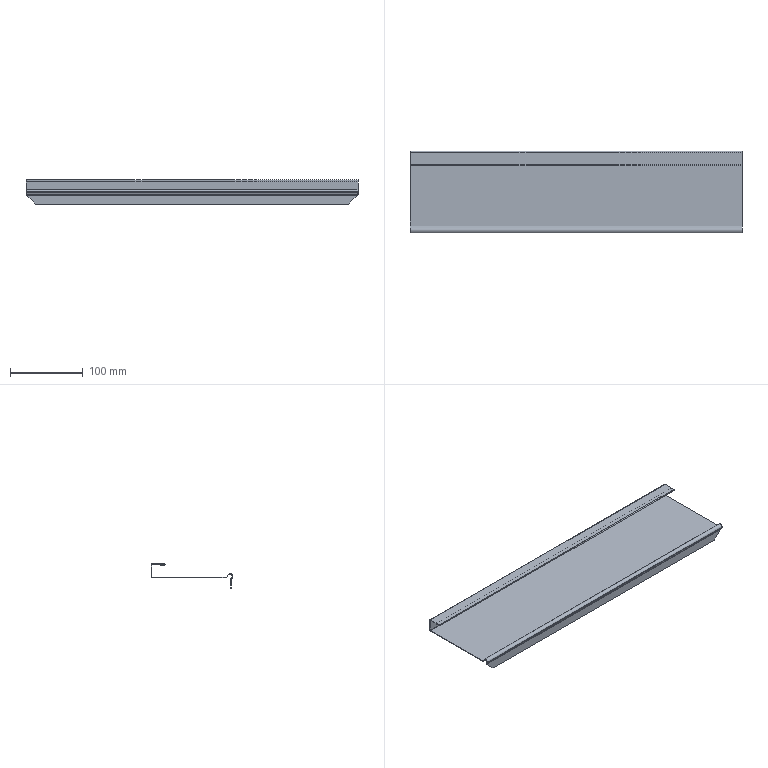Part | SolidWorks | features SM3dBend 4, EdgeFlange 2, FlatPattern 1, Hem 1, SMBaseFlange 1, SheetMetal 1 | 1 solid | 65 faces | box 455 x 111.371 x 33.2 mm | volume 63198 mm3 | plane 48 | cylinder 14 | spline 3 | commonest cylinder face diameters 1 x3 2.6 x3 0.1 x1 1.2 x1 1.7 x1 2.8 x1